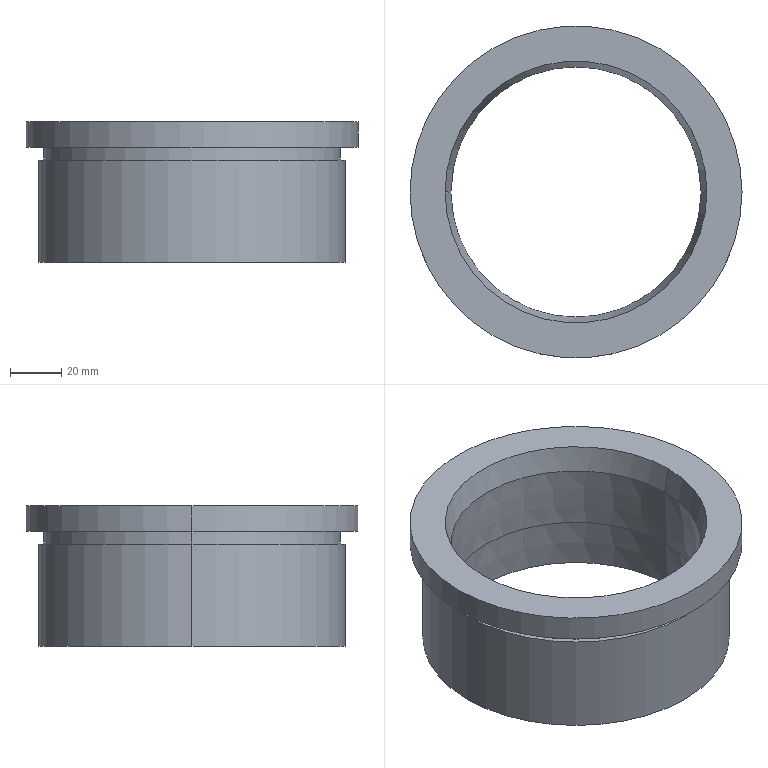Part | SolidWorks | features Revolution 1 | 1 solid | 16 faces | box 130 x 130 x 55 mm | volume 211427 mm3 | cone 6 | cylinder 6 | plane 4 | commonest cylinder face diameters 116 x2 120 x2 130 x2
STEP:
#1=CARTESIAN_POINT('',(472.231,234.744,-1054.693));
#2=VERTEX_POINT('',#1);
#3=CARTESIAN_POINT('',(570.231,234.744,-1054.693));
#4=VERTEX_POINT('',#3);
#5=CARTESIAN_POINT('',(521.231,234.744,-1054.693));
#6=DIRECTION('',(0.,0.,1.));
#7=DIRECTION('',(1.,0.,0.));
#8=AXIS2_PLACEMENT_3D('',#5,#6,#7);
#9=CIRCLE('',#8,49.);
#10=EDGE_CURVE('',#2,#4,#9,.T.);
#11=ORIENTED_EDGE('',*,*,#10,.F.);
#12=CARTESIAN_POINT('',(469.981,234.744,-1044.693));
#13=VERTEX_POINT('',#12);
#14=CARTESIAN_POINT('',(472.231,234.744,-1054.693));
#15=DIRECTION('',(-0.2195,0.,0.9756));
#16=VECTOR('',#15,1000.);
#17=LINE('',#14,#16);
#18=EDGE_CURVE('',#2,#13,#17,.T.);
#19=ORIENTED_EDGE('',*,*,#18,.T.);
#20=CARTESIAN_POINT('',(572.481,234.744,-1044.693));
#21=VERTEX_POINT('',#20);
#22=CARTESIAN_POINT('',(521.231,234.744,-1044.693));
#23=DIRECTION('',(0.,0.,1.));
#24=DIRECTION('',(1.,0.,0.));
#25=AXIS2_PLACEMENT_3D('',#22,#23,#24);
#26=CIRCLE('',#25,51.25);
#27=EDGE_CURVE('',#13,#21,#26,.T.);
#28=ORIENTED_EDGE('',*,*,#27,.T.);
#29=CARTESIAN_POINT('',(570.231,234.744,-1054.693));
#30=DIRECTION('',(0.2195,0.,0.9756));
#31=VECTOR('',#30,1000.);
#32=LINE('',#29,#31);
#33=EDGE_CURVE('',#4,#21,#32,.T.);
#34=ORIENTED_EDGE('',*,*,#33,.F.);
#35=EDGE_LOOP('',(#11,#19,#28,#34));
#36=FACE_OUTER_BOUND('',#35,.T.);
#37=CARTESIAN_POINT('',(521.231,234.744,-1054.693));
#38=DIRECTION('',(0.,0.,1.));
#39=DIRECTION('',(1.,0.,0.));
#40=AXIS2_PLACEMENT_3D('',#37,#38,#39);
#41=CONICAL_SURFACE('',#40,49.,0.2213);
#42=ADVANCED_FACE('',(#36),#41,.F.);
#43=ORIENTED_EDGE('',*,*,#10,.T.);
#44=CARTESIAN_POINT('',(570.731,234.744,-1079.693));
#45=VERTEX_POINT('',#44);
#46=CARTESIAN_POINT('',(570.731,234.744,-1079.693));
#47=DIRECTION('',(0.02,0.,-0.9998));
#48=VECTOR('',#47,1000.);
#49=LINE('',#46,#48);
#50=EDGE_CURVE('',#4,#45,#49,.T.);
#51=ORIENTED_EDGE('',*,*,#50,.T.);
#52=CARTESIAN_POINT('',(471.731,234.744,-1079.693));
#53=VERTEX_POINT('',#52);
#54=CARTESIAN_POINT('',(521.231,234.744,-1079.693));
#55=DIRECTION('',(0.,0.,1.));
#56=DIRECTION('',(1.,0.,0.));
#57=AXIS2_PLACEMENT_3D('',#54,#55,#56);
#58=CIRCLE('',#57,49.5);
#59=EDGE_CURVE('',#53,#45,#58,.T.);
#60=ORIENTED_EDGE('',*,*,#59,.F.);
#61=CARTESIAN_POINT('',(471.731,234.744,-1079.693));
#62=DIRECTION('',(-0.02,0.,-0.9998));
#63=VECTOR('',#62,1000.);
#64=LINE('',#61,#63);
#65=EDGE_CURVE('',#2,#53,#64,.T.);
#66=ORIENTED_EDGE('',*,*,#65,.F.);
#67=EDGE_LOOP('',(#43,#51,#60,#66));
#68=FACE_OUTER_BOUND('',#67,.T.);
#69=CARTESIAN_POINT('',(521.231,234.744,-1079.693));
#70=DIRECTION('',(0.,0.,-1.));
#71=DIRECTION('',(-1.,0.,0.));
#72=AXIS2_PLACEMENT_3D('',#69,#70,#71);
#73=CONICAL_SURFACE('',#72,49.5,0.02);
#74=ADVANCED_FACE('',(#68),#73,.F.);
#75=ORIENTED_EDGE('',*,*,#59,.T.);
#76=CARTESIAN_POINT('',(571.731,234.744,-1099.693));
#77=VERTEX_POINT('',#76);
#78=CARTESIAN_POINT('',(571.731,234.744,-1099.693));
#79=DIRECTION('',(0.04994,0.,-0.9988));
#80=VECTOR('',#79,1000.);
#81=LINE('',#78,#80);
#82=EDGE_CURVE('',#45,#77,#81,.T.);
#83=ORIENTED_EDGE('',*,*,#82,.T.);
#84=CARTESIAN_POINT('',(470.731,234.744,-1099.693));
#85=VERTEX_POINT('',#84);
#86=CARTESIAN_POINT('',(521.231,234.744,-1099.693));
#87=DIRECTION('',(0.,0.,1.));
#88=DIRECTION('',(1.,0.,0.));
#89=AXIS2_PLACEMENT_3D('',#86,#87,#88);
#90=CIRCLE('',#89,50.5);
#91=EDGE_CURVE('',#85,#77,#90,.T.);
#92=ORIENTED_EDGE('',*,*,#91,.F.);
#93=CARTESIAN_POINT('',(470.731,234.744,-1099.693));
#94=DIRECTION('',(-0.04994,0.,-0.9988));
#95=VECTOR('',#94,1000.);
#96=LINE('',#93,#95);
#97=EDGE_CURVE('',#53,#85,#96,.T.);
#98=ORIENTED_EDGE('',*,*,#97,.F.);
#99=EDGE_LOOP('',(#75,#83,#92,#98));
#100=FACE_OUTER_BOUND('',#99,.T.);
#101=CARTESIAN_POINT('',(521.231,234.744,-1099.693));
#102=DIRECTION('',(0.,0.,-1.));
#103=DIRECTION('',(-1.,0.,0.));
#104=AXIS2_PLACEMENT_3D('',#101,#102,#103);
#105=CONICAL_SURFACE('',#104,50.5,0.04996);
#106=ADVANCED_FACE('',(#100),#105,.F.);
#107=CARTESIAN_POINT('',(581.231,234.744,-1099.693));
#108=VERTEX_POINT('',#107);
#109=CARTESIAN_POINT('',(461.231,234.744,-1099.693));
#110=VERTEX_POINT('',#109);
#111=CARTESIAN_POINT('',(521.231,234.744,-1099.693));
#112=DIRECTION('',(0.,0.,1.));
#113=DIRECTION('',(1.,0.,0.));
#114=AXIS2_PLACEMENT_3D('',#111,#112,#113);
#115=CIRCLE('',#114,60.);
#116=EDGE_CURVE('',#108,#110,#115,.T.);
#117=ORIENTED_EDGE('',*,*,#116,.T.);
#118=CARTESIAN_POINT('',(461.231,234.744,-1059.693));
#119=VERTEX_POINT('',#118);
#120=CARTESIAN_POINT('',(461.231,234.744,-1099.693));
#121=DIRECTION('',(0.,0.,1.));
#122=VECTOR('',#121,1000.);
#123=LINE('',#120,#122);
#124=EDGE_CURVE('',#110,#119,#123,.T.);
#125=ORIENTED_EDGE('',*,*,#124,.T.);
#126=CARTESIAN_POINT('',(581.231,234.744,-1059.693));
#127=VERTEX_POINT('',#126);
#128=CARTESIAN_POINT('',(521.231,234.744,-1059.693));
#129=DIRECTION('',(0.,0.,1.));
#130=DIRECTION('',(1.,0.,0.));
#131=AXIS2_PLACEMENT_3D('',#128,#129,#130);
#132=CIRCLE('',#131,60.);
#133=EDGE_CURVE('',#127,#119,#132,.T.);
#134=ORIENTED_EDGE('',*,*,#133,.F.);
#135=CARTESIAN_POINT('',(581.231,234.744,-1099.693));
#136=DIRECTION('',(0.,0.,1.));
#137=VECTOR('',#136,1000.);
#138=LINE('',#135,#137);
#139=EDGE_CURVE('',#108,#127,#138,.T.);
#140=ORIENTED_EDGE('',*,*,#139,.F.);
#141=EDGE_LOOP('',(#117,#125,#134,#140));
#142=FACE_OUTER_BOUND('',#141,.T.);
#143=CARTESIAN_POINT('',(521.231,234.744,-1099.693));
#144=DIRECTION('',(0.,0.,1.));
#145=DIRECTION('',(1.,0.,0.));
#146=AXIS2_PLACEMENT_3D('',#143,#144,#145);
#147=CYLINDRICAL_SURFACE('',#146,60.);
#148=ADVANCED_FACE('',(#142),#147,.T.);
#149=CARTESIAN_POINT('',(579.231,234.744,-1059.693));
#150=VERTEX_POINT('',#149);
#151=CARTESIAN_POINT('',(463.231,234.744,-1059.693));
#152=VERTEX_POINT('',#151);
#153=CARTESIAN_POINT('',(521.231,234.744,-1059.693));
#154=DIRECTION('',(0.,0.,1.));
#155=DIRECTION('',(1.,0.,0.));
#156=AXIS2_PLACEMENT_3D('',#153,#154,#155);
#157=CIRCLE('',#156,58.);
#158=EDGE_CURVE('',#150,#152,#157,.T.);
#159=ORIENTED_EDGE('',*,*,#158,.T.);
#160=CARTESIAN_POINT('',(463.231,234.744,-1054.693));
#161=VERTEX_POINT('',#160);
#162=CARTESIAN_POINT('',(463.231,234.744,-1099.693));
#163=DIRECTION('',(0.,0.,1.));
#164=VECTOR('',#163,1000.);
#165=LINE('',#162,#164);
#166=EDGE_CURVE('',#152,#161,#165,.T.);
#167=ORIENTED_EDGE('',*,*,#166,.T.);
#168=CARTESIAN_POINT('',(579.231,234.744,-1054.693));
#169=VERTEX_POINT('',#168);
#170=CARTESIAN_POINT('',(521.231,234.744,-1054.693));
#171=DIRECTION('',(0.,0.,1.));
#172=DIRECTION('',(1.,0.,0.));
#173=AXIS2_PLACEMENT_3D('',#170,#171,#172);
#174=CIRCLE('',#173,58.);
#175=EDGE_CURVE('',#169,#161,#174,.T.);
#176=ORIENTED_EDGE('',*,*,#175,.F.);
#177=CARTESIAN_POINT('',(579.231,234.744,-1099.693));
#178=DIRECTION('',(0.,0.,1.));
#179=VECTOR('',#178,1000.);
#180=LINE('',#177,#179);
#181=EDGE_CURVE('',#150,#169,#180,.T.);
#182=ORIENTED_EDGE('',*,*,#181,.F.);
#183=EDGE_LOOP('',(#159,#167,#176,#182));
#184=FACE_OUTER_BOUND('',#183,.T.);
#185=CARTESIAN_POINT('',(521.231,234.744,-1099.693));
#186=DIRECTION('',(0.,0.,1.));
#187=DIRECTION('',(1.,0.,0.));
#188=AXIS2_PLACEMENT_3D('',#185,#186,#187);
#189=CYLINDRICAL_SURFACE('',#188,58.);
#190=ADVANCED_FACE('',(#184),#189,.T.);
#191=CARTESIAN_POINT('',(586.231,234.744,-1054.693));
#192=VERTEX_POINT('',#191);
#193=CARTESIAN_POINT('',(456.231,234.744,-1054.693));
#194=VERTEX_POINT('',#193);
#195=CARTESIAN_POINT('',(521.231,234.744,-1054.693));
#196=DIRECTION('',(0.,0.,1.));
#197=DIRECTION('',(1.,0.,0.));
#198=AXIS2_PLACEMENT_3D('',#195,#196,#197);
#199=CIRCLE('',#198,65.);
#200=EDGE_CURVE('',#192,#194,#199,.T.);
#201=ORIENTED_EDGE('',*,*,#200,.T.);
#202=CARTESIAN_POINT('',(456.231,234.744,-1044.693));
#203=VERTEX_POINT('',#202);
#204=CARTESIAN_POINT('',(456.231,234.744,-1099.693));
#205=DIRECTION('',(0.,0.,1.));
#206=VECTOR('',#205,1000.);
#207=LINE('',#204,#206);
#208=EDGE_CURVE('',#194,#203,#207,.T.);
#209=ORIENTED_EDGE('',*,*,#208,.T.);
#210=CARTESIAN_POINT('',(586.231,234.744,-1044.693));
#211=VERTEX_POINT('',#210);
#212=CARTESIAN_POINT('',(521.231,234.744,-1044.693));
#213=DIRECTION('',(0.,0.,1.));
#214=DIRECTION('',(1.,0.,0.));
#215=AXIS2_PLACEMENT_3D('',#212,#213,#214);
#216=CIRCLE('',#215,65.);
#217=EDGE_CURVE('',#211,#203,#216,.T.);
#218=ORIENTED_EDGE('',*,*,#217,.F.);
#219=CARTESIAN_POINT('',(586.231,234.744,-1099.693));
#220=DIRECTION('',(0.,0.,1.));
#221=VECTOR('',#220,1000.);
#222=LINE('',#219,#221);
#223=EDGE_CURVE('',#192,#211,#222,.T.);
#224=ORIENTED_EDGE('',*,*,#223,.F.);
#225=EDGE_LOOP('',(#201,#209,#218,#224));
#226=FACE_OUTER_BOUND('',#225,.T.);
#227=CARTESIAN_POINT('',(521.231,234.744,-1099.693));
#228=DIRECTION('',(0.,0.,1.));
#229=DIRECTION('',(1.,0.,0.));
#230=AXIS2_PLACEMENT_3D('',#227,#228,#229);
#231=CYLINDRICAL_SURFACE('',#230,65.);
#232=ADVANCED_FACE('',(#226),#231,.T.);
#233=ORIENTED_EDGE('',*,*,#208,.F.);
#234=CARTESIAN_POINT('',(521.231,234.744,-1054.693));
#235=DIRECTION('',(0.,0.,1.));
#236=DIRECTION('',(1.,0.,0.));
#237=AXIS2_PLACEMENT_3D('',#234,#235,#236);
#238=CIRCLE('',#237,65.);
#239=EDGE_CURVE('',#194,#192,#238,.T.);
#240=ORIENTED_EDGE('',*,*,#239,.T.);
#241=ORIENTED_EDGE('',*,*,#223,.T.);
#242=CARTESIAN_POINT('',(521.231,234.744,-1044.693));
#243=DIRECTION('',(0.,0.,1.));
#244=DIRECTION('',(1.,0.,0.));
#245=AXIS2_PLACEMENT_3D('',#242,#243,#244);
#246=CIRCLE('',#245,65.);
#247=EDGE_CURVE('',#203,#211,#246,.T.);
#248=ORIENTED_EDGE('',*,*,#247,.F.);
#249=EDGE_LOOP('',(#233,#240,#241,#248));
#250=FACE_OUTER_BOUND('',#249,.T.);
#251=CARTESIAN_POINT('',(521.231,234.744,-1099.693));
#252=DIRECTION('',(0.,0.,1.));
#253=DIRECTION('',(1.,0.,0.));
#254=AXIS2_PLACEMENT_3D('',#251,#252,#253);
#255=CYLINDRICAL_SURFACE('',#254,65.);
#256=ADVANCED_FACE('',(#250),#255,.T.);
#257=ORIENTED_EDGE('',*,*,#175,.T.);
#258=CARTESIAN_POINT('',(521.231,234.744,-1054.693));
#259=DIRECTION('',(0.,0.,1.));
#260=DIRECTION('',(1.,0.,0.));
#261=AXIS2_PLACEMENT_3D('',#258,#259,#260);
#262=CIRCLE('',#261,58.);
#263=EDGE_CURVE('',#161,#169,#262,.T.);
#264=ORIENTED_EDGE('',*,*,#263,.T.);
#265=EDGE_LOOP('',(#257,#264));
#266=FACE_BOUND('',#265,.T.);
#267=ORIENTED_EDGE('',*,*,#200,.F.);
#268=ORIENTED_EDGE('',*,*,#239,.F.);
#269=EDGE_LOOP('',(#267,#268));
#270=FACE_OUTER_BOUND('',#269,.T.);
#271=CARTESIAN_POINT('',(586.231,234.744,-1054.693));
#272=DIRECTION('',(0.,0.,-1.));
#273=DIRECTION('',(-1.,0.,0.));
#274=AXIS2_PLACEMENT_3D('',#271,#272,#273);
#275=PLANE('',#274);
#276=ADVANCED_FACE('',(#266,#270),#275,.T.);
#277=ORIENTED_EDGE('',*,*,#166,.F.);
#278=CARTESIAN_POINT('',(521.231,234.744,-1059.693));
#279=DIRECTION('',(0.,0.,1.));
#280=DIRECTION('',(1.,0.,0.));
#281=AXIS2_PLACEMENT_3D('',#278,#279,#280);
#282=CIRCLE('',#281,58.);
#283=EDGE_CURVE('',#152,#150,#282,.T.);
#284=ORIENTED_EDGE('',*,*,#283,.T.);
#285=ORIENTED_EDGE('',*,*,#181,.T.);
#286=ORIENTED_EDGE('',*,*,#263,.F.);
#287=EDGE_LOOP('',(#277,#284,#285,#286));
#288=FACE_OUTER_BOUND('',#287,.T.);
#289=CARTESIAN_POINT('',(521.231,234.744,-1099.693));
#290=DIRECTION('',(0.,0.,1.));
#291=DIRECTION('',(1.,0.,0.));
#292=AXIS2_PLACEMENT_3D('',#289,#290,#291);
#293=CYLINDRICAL_SURFACE('',#292,58.);
#294=ADVANCED_FACE('',(#288),#293,.T.);
#295=ORIENTED_EDGE('',*,*,#133,.T.);
#296=CARTESIAN_POINT('',(521.231,234.744,-1059.693));
#297=DIRECTION('',(0.,0.,1.));
#298=DIRECTION('',(1.,0.,0.));
#299=AXIS2_PLACEMENT_3D('',#296,#297,#298);
#300=CIRCLE('',#299,60.);
#301=EDGE_CURVE('',#119,#127,#300,.T.);
#302=ORIENTED_EDGE('',*,*,#301,.T.);
#303=EDGE_LOOP('',(#295,#302));
#304=FACE_OUTER_BOUND('',#303,.T.);
#305=ORIENTED_EDGE('',*,*,#158,.F.);
#306=ORIENTED_EDGE('',*,*,#283,.F.);
#307=EDGE_LOOP('',(#305,#306));
#308=FACE_BOUND('',#307,.T.);
#309=CARTESIAN_POINT('',(579.231,234.744,-1059.693));
#310=DIRECTION('',(0.,0.,1.));
#311=DIRECTION('',(1.,0.,0.));
#312=AXIS2_PLACEMENT_3D('',#309,#310,#311);
#313=PLANE('',#312);
#314=ADVANCED_FACE('',(#304,#308),#313,.T.);
#315=ORIENTED_EDGE('',*,*,#124,.F.);
#316=CARTESIAN_POINT('',(521.231,234.744,-1099.693));
#317=DIRECTION('',(0.,0.,1.));
#318=DIRECTION('',(1.,0.,0.));
#319=AXIS2_PLACEMENT_3D('',#316,#317,#318);
#320=CIRCLE('',#319,60.);
#321=EDGE_CURVE('',#110,#108,#320,.T.);
#322=ORIENTED_EDGE('',*,*,#321,.T.);
#323=ORIENTED_EDGE('',*,*,#139,.T.);
#324=ORIENTED_EDGE('',*,*,#301,.F.);
#325=EDGE_LOOP('',(#315,#322,#323,#324));
#326=FACE_OUTER_BOUND('',#325,.T.);
#327=CARTESIAN_POINT('',(521.231,234.744,-1099.693));
#328=DIRECTION('',(0.,0.,1.));
#329=DIRECTION('',(1.,0.,0.));
#330=AXIS2_PLACEMENT_3D('',#327,#328,#329);
#331=CYLINDRICAL_SURFACE('',#330,60.);
#332=ADVANCED_FACE('',(#326),#331,.T.);
#333=ORIENTED_EDGE('',*,*,#91,.T.);
#334=CARTESIAN_POINT('',(521.231,234.744,-1099.693));
#335=DIRECTION('',(0.,0.,1.));
#336=DIRECTION('',(1.,0.,0.));
#337=AXIS2_PLACEMENT_3D('',#334,#335,#336);
#338=CIRCLE('',#337,50.5);
#339=EDGE_CURVE('',#77,#85,#338,.T.);
#340=ORIENTED_EDGE('',*,*,#339,.T.);
#341=EDGE_LOOP('',(#333,#340));
#342=FACE_BOUND('',#341,.T.);
#343=ORIENTED_EDGE('',*,*,#116,.F.);
#344=ORIENTED_EDGE('',*,*,#321,.F.);
#345=EDGE_LOOP('',(#343,#344));
#346=FACE_OUTER_BOUND('',#345,.T.);
#347=CARTESIAN_POINT('',(581.231,234.744,-1099.693));
#348=DIRECTION('',(0.,0.,-1.));
#349=DIRECTION('',(-1.,0.,0.));
#350=AXIS2_PLACEMENT_3D('',#347,#348,#349);
#351=PLANE('',#350);
#352=ADVANCED_FACE('',(#342,#346),#351,.T.);
#353=ORIENTED_EDGE('',*,*,#82,.F.);
#354=CARTESIAN_POINT('',(521.231,234.744,-1079.693));
#355=DIRECTION('',(0.,0.,1.));
#356=DIRECTION('',(1.,0.,0.));
#357=AXIS2_PLACEMENT_3D('',#354,#355,#356);
#358=CIRCLE('',#357,49.5);
#359=EDGE_CURVE('',#45,#53,#358,.T.);
#360=ORIENTED_EDGE('',*,*,#359,.T.);
#361=ORIENTED_EDGE('',*,*,#97,.T.);
#362=ORIENTED_EDGE('',*,*,#339,.F.);
#363=EDGE_LOOP('',(#353,#360,#361,#362));
#364=FACE_OUTER_BOUND('',#363,.T.);
#365=CARTESIAN_POINT('',(521.231,234.744,-1099.693));
#366=DIRECTION('',(0.,0.,-1.));
#367=DIRECTION('',(-1.,0.,0.));
#368=AXIS2_PLACEMENT_3D('',#365,#366,#367);
#369=CONICAL_SURFACE('',#368,50.5,0.04996);
#370=ADVANCED_FACE('',(#364),#369,.F.);
#371=ORIENTED_EDGE('',*,*,#50,.F.);
#372=CARTESIAN_POINT('',(521.231,234.744,-1054.693));
#373=DIRECTION('',(0.,0.,1.));
#374=DIRECTION('',(1.,0.,0.));
#375=AXIS2_PLACEMENT_3D('',#372,#373,#374);
#376=CIRCLE('',#375,49.);
#377=EDGE_CURVE('',#4,#2,#376,.T.);
#378=ORIENTED_EDGE('',*,*,#377,.T.);
#379=ORIENTED_EDGE('',*,*,#65,.T.);
#380=ORIENTED_EDGE('',*,*,#359,.F.);
#381=EDGE_LOOP('',(#371,#378,#379,#380));
#382=FACE_OUTER_BOUND('',#381,.T.);
#383=CARTESIAN_POINT('',(521.231,234.744,-1079.693));
#384=DIRECTION('',(0.,0.,-1.));
#385=DIRECTION('',(-1.,0.,0.));
#386=AXIS2_PLACEMENT_3D('',#383,#384,#385);
#387=CONICAL_SURFACE('',#386,49.5,0.02);
#388=ADVANCED_FACE('',(#382),#387,.F.);
#389=ORIENTED_EDGE('',*,*,#18,.F.);
#390=ORIENTED_EDGE('',*,*,#377,.F.);
#391=ORIENTED_EDGE('',*,*,#33,.T.);
#392=CARTESIAN_POINT('',(521.231,234.744,-1044.693));
#393=DIRECTION('',(0.,0.,1.));
#394=DIRECTION('',(1.,0.,0.));
#395=AXIS2_PLACEMENT_3D('',#392,#393,#394);
#396=CIRCLE('',#395,51.25);
#397=EDGE_CURVE('',#21,#13,#396,.T.);
#398=ORIENTED_EDGE('',*,*,#397,.T.);
#399=EDGE_LOOP('',(#389,#390,#391,#398));
#400=FACE_OUTER_BOUND('',#399,.T.);
#401=CARTESIAN_POINT('',(521.231,234.744,-1054.693));
#402=DIRECTION('',(0.,0.,1.));
#403=DIRECTION('',(1.,0.,0.));
#404=AXIS2_PLACEMENT_3D('',#401,#402,#403);
#405=CONICAL_SURFACE('',#404,49.,0.2213);
#406=ADVANCED_FACE('',(#400),#405,.F.);
#407=ORIENTED_EDGE('',*,*,#217,.T.);
#408=ORIENTED_EDGE('',*,*,#247,.T.);
#409=EDGE_LOOP('',(#407,#408));
#410=FACE_OUTER_BOUND('',#409,.T.);
#411=ORIENTED_EDGE('',*,*,#397,.F.);
#412=ORIENTED_EDGE('',*,*,#27,.F.);
#413=EDGE_LOOP('',(#411,#412));
#414=FACE_BOUND('',#413,.T.);
#415=CARTESIAN_POINT('',(572.481,234.744,-1044.693));
#416=DIRECTION('',(0.,0.,1.));
#417=DIRECTION('',(1.,0.,0.));
#418=AXIS2_PLACEMENT_3D('',#415,#416,#417);
#419=PLANE('',#418);
#420=ADVANCED_FACE('',(#410,#414),#419,.T.);
#421=CLOSED_SHELL('',(#42,#74,#106,#148,#190,#232,#256,#276,#294,#314,#332,#352,#370,#388,#406,#420));
#422=MANIFOLD_SOLID_BREP('',#421);
#423=CARTESIAN_POINT('',(0.,0.,0.));
#424=DIRECTION('',(0.,0.,1.));
#425=DIRECTION('',(1.,0.,0.));
#426=AXIS2_PLACEMENT_3D('',#423,#424,#425);
#427=(LENGTH_UNIT()NAMED_UNIT(*)SI_UNIT(.MILLI.,.METRE.));
#428=UNCERTAINTY_MEASURE_WITH_UNIT(LENGTH_MEASURE(0.00001),#427,'','');
#429=(NAMED_UNIT(*)PLANE_ANGLE_UNIT()SI_UNIT($,.RADIAN.));
#430=(NAMED_UNIT(*)SI_UNIT($,.STERADIAN.)SOLID_ANGLE_UNIT());
#431=(GEOMETRIC_REPRESENTATION_CONTEXT(3)GLOBAL_UNCERTAINTY_ASSIGNED_CONTEXT((#428))GLOBAL_UNIT_ASSIGNED_CONTEXT((#427,#429,#430))REPRESENTATION_CONTEXT('',''));
#432=ADVANCED_BREP_SHAPE_REPRESENTATION('',(#422,#426),#431);